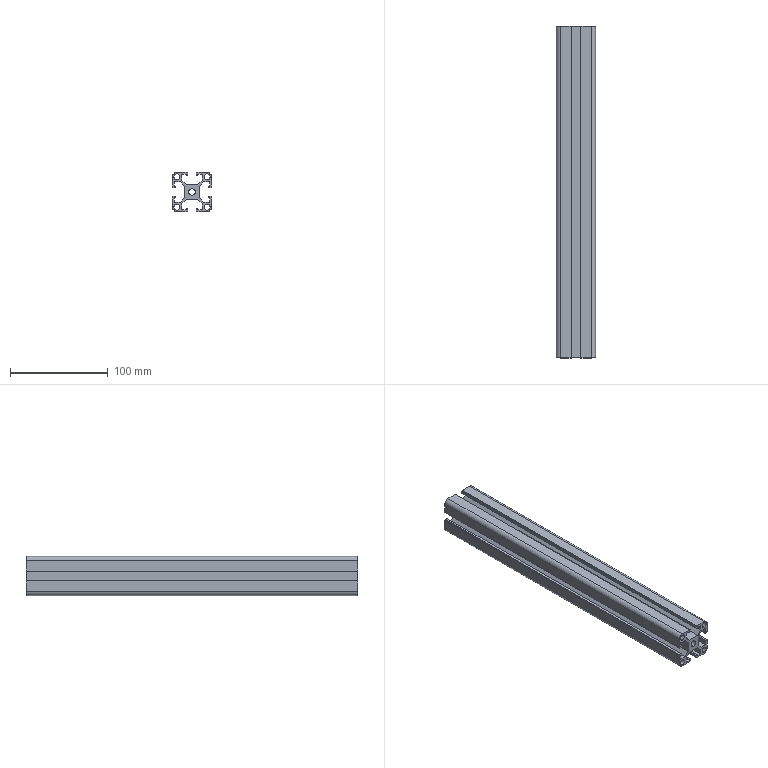Part | SolidWorks | features HoleWzd 1, WeldMemberFeat 1, WeldmentFeature 1 | 1 solid | 96 faces | box 40 x 340 x 40 mm | volume 205625 mm3 | plane 78 | cylinder 16 | cone 2 | commonest cylinder face diameters 6 x8 9 x4 6.8 x2 6.9 x2